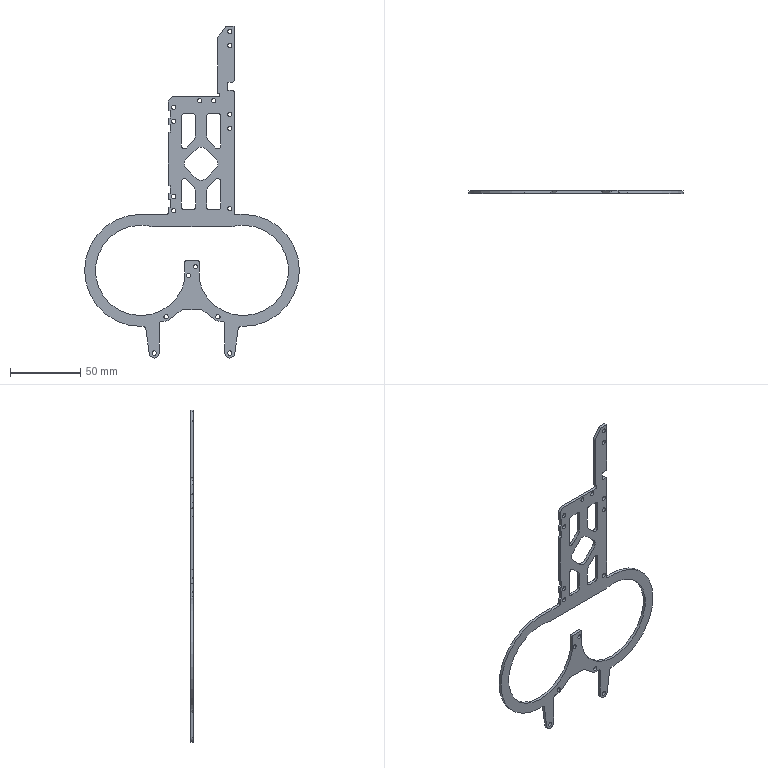Part | SolidWorks | features Fillet 4, ICE 3, Chamfer 1, Extrusion 1 | 1 solid | 164 faces | box 153.25 x 2 x 236.9 mm | volume 13689 mm3 | cylinder 98 | plane 66 | commonest cylinder face diameters 3.1 x34 4 x24 10 x11 1 x8 2 x8 64.5 x6